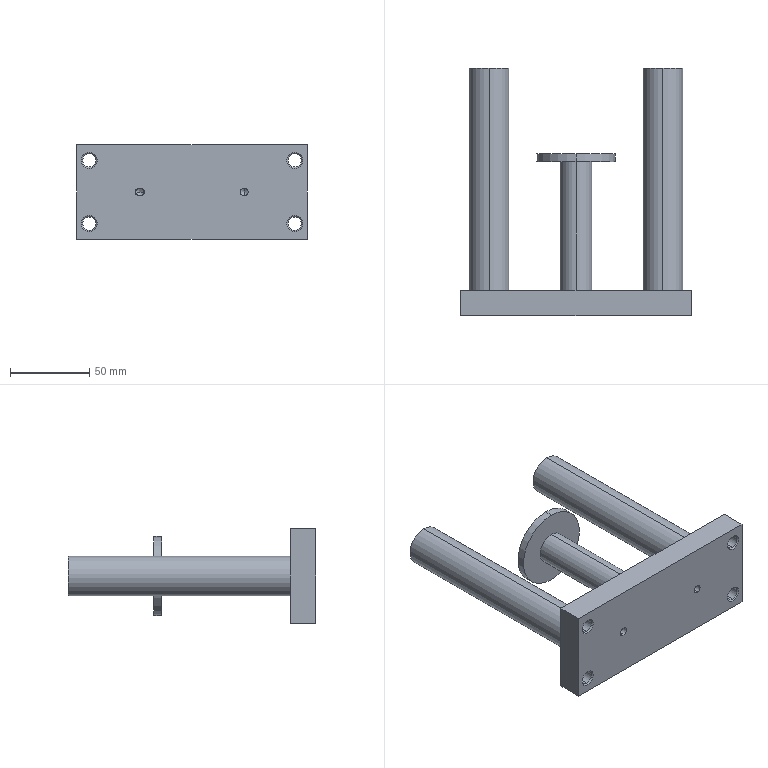Part | SolidWorks | features BaseBody 1 | 1 solid | 56 faces | box 146 x 156.5 x 60 mm | volume 309564 mm3 | cylinder 22 | cone 20 | plane 14 | commonest cylinder face diameters 8.376 x8 5 x6 25 x4 20 x2 50 x2
STEP:
#1=CARTESIAN_POINT('',(33.,107.,140.621));
#2=VERTEX_POINT('',#1);
#3=CARTESIAN_POINT('',(33.,107.,145.621));
#4=VERTEX_POINT('',#3);
#5=CARTESIAN_POINT('',(33.,107.,143.121));
#6=DIRECTION('',(0.,1.,0.));
#7=DIRECTION('',(0.,0.,1.));
#8=AXIS2_PLACEMENT_3D('',#5,#6,#7);
#9=CIRCLE('',#8,2.5);
#10=EDGE_CURVE('',#2,#4,#9,.T.);
#11=ORIENTED_EDGE('',*,*,#10,.F.);
#12=CARTESIAN_POINT('',(33.,115.,140.621));
#13=VERTEX_POINT('',#12);
#14=CARTESIAN_POINT('',(33.,111.,140.621));
#15=DIRECTION('',(0.,1.,0.));
#16=VECTOR('',#15,1000.);
#17=LINE('',#14,#16);
#18=EDGE_CURVE('',#2,#13,#17,.T.);
#19=ORIENTED_EDGE('',*,*,#18,.T.);
#20=CARTESIAN_POINT('',(33.,115.,145.621));
#21=VERTEX_POINT('',#20);
#22=CARTESIAN_POINT('',(33.,115.,143.121));
#23=DIRECTION('',(0.,-1.,0.));
#24=DIRECTION('',(0.,0.,1.));
#25=AXIS2_PLACEMENT_3D('',#22,#23,#24);
#26=CIRCLE('',#25,2.5);
#27=EDGE_CURVE('',#21,#13,#26,.T.);
#28=ORIENTED_EDGE('',*,*,#27,.F.);
#29=CARTESIAN_POINT('',(33.,111.,145.621));
#30=DIRECTION('',(0.,1.,0.));
#31=VECTOR('',#30,1000.);
#32=LINE('',#29,#31);
#33=EDGE_CURVE('',#4,#21,#32,.T.);
#34=ORIENTED_EDGE('',*,*,#33,.F.);
#35=EDGE_LOOP('',(#11,#19,#28,#34));
#36=FACE_OUTER_BOUND('',#35,.T.);
#37=CARTESIAN_POINT('',(33.,111.,143.121));
#38=DIRECTION('',(0.,1.,0.));
#39=DIRECTION('',(0.,0.,1.));
#40=AXIS2_PLACEMENT_3D('',#37,#38,#39);
#41=CYLINDRICAL_SURFACE('',#40,2.5);
#42=ADVANCED_FACE('',(#36),#41,.F.);
#43=CARTESIAN_POINT('',(65.,107.812,127.309));
#44=VERTEX_POINT('',#43);
#45=CARTESIAN_POINT('',(65.,107.812,118.933));
#46=VERTEX_POINT('',#45);
#47=CARTESIAN_POINT('',(65.,107.812,123.121));
#48=DIRECTION('',(0.,-1.,0.));
#49=DIRECTION('',(0.,0.,-1.));
#50=AXIS2_PLACEMENT_3D('',#47,#48,#49);
#51=CIRCLE('',#50,4.188);
#52=EDGE_CURVE('',#44,#46,#51,.T.);
#53=ORIENTED_EDGE('',*,*,#52,.F.);
#54=CARTESIAN_POINT('',(65.,107.,128.121));
#55=VERTEX_POINT('',#54);
#56=CARTESIAN_POINT('',(65.,107.,128.121));
#57=DIRECTION('',(0.,-0.7071,0.7071));
#58=VECTOR('',#57,1000.);
#59=LINE('',#56,#58);
#60=EDGE_CURVE('',#44,#55,#59,.T.);
#61=ORIENTED_EDGE('',*,*,#60,.T.);
#62=CARTESIAN_POINT('',(65.,107.,118.121));
#63=VERTEX_POINT('',#62);
#64=CARTESIAN_POINT('',(65.,107.,123.121));
#65=DIRECTION('',(0.,1.,0.));
#66=DIRECTION('',(0.,0.,-1.));
#67=AXIS2_PLACEMENT_3D('',#64,#65,#66);
#68=CIRCLE('',#67,5.);
#69=EDGE_CURVE('',#63,#55,#68,.T.);
#70=ORIENTED_EDGE('',*,*,#69,.F.);
#71=CARTESIAN_POINT('',(65.,107.,118.121));
#72=DIRECTION('',(0.,-0.7071,-0.7071));
#73=VECTOR('',#72,1000.);
#74=LINE('',#71,#73);
#75=EDGE_CURVE('',#46,#63,#74,.T.);
#76=ORIENTED_EDGE('',*,*,#75,.F.);
#77=EDGE_LOOP('',(#53,#61,#70,#76));
#78=FACE_OUTER_BOUND('',#77,.T.);
#79=CARTESIAN_POINT('',(65.,107.,123.121));
#80=DIRECTION('',(0.,-1.,0.));
#81=DIRECTION('',(0.,0.,-1.));
#82=AXIS2_PLACEMENT_3D('',#79,#80,#81);
#83=CONICAL_SURFACE('',#82,5.,0.7854);
#84=ADVANCED_FACE('',(#78),#83,.F.);
#85=CARTESIAN_POINT('',(65.,107.812,167.309));
#86=VERTEX_POINT('',#85);
#87=CARTESIAN_POINT('',(65.,107.812,158.933));
#88=VERTEX_POINT('',#87);
#89=CARTESIAN_POINT('',(65.,107.812,163.121));
#90=DIRECTION('',(0.,-1.,0.));
#91=DIRECTION('',(0.,0.,-1.));
#92=AXIS2_PLACEMENT_3D('',#89,#90,#91);
#93=CIRCLE('',#92,4.188);
#94=EDGE_CURVE('',#86,#88,#93,.T.);
#95=ORIENTED_EDGE('',*,*,#94,.F.);
#96=CARTESIAN_POINT('',(65.,107.,168.121));
#97=VERTEX_POINT('',#96);
#98=CARTESIAN_POINT('',(65.,107.,168.121));
#99=DIRECTION('',(0.,-0.7071,0.7071));
#100=VECTOR('',#99,1000.);
#101=LINE('',#98,#100);
#102=EDGE_CURVE('',#86,#97,#101,.T.);
#103=ORIENTED_EDGE('',*,*,#102,.T.);
#104=CARTESIAN_POINT('',(65.,107.,158.121));
#105=VERTEX_POINT('',#104);
#106=CARTESIAN_POINT('',(65.,107.,163.121));
#107=DIRECTION('',(0.,1.,0.));
#108=DIRECTION('',(0.,0.,-1.));
#109=AXIS2_PLACEMENT_3D('',#106,#107,#108);
#110=CIRCLE('',#109,5.);
#111=EDGE_CURVE('',#105,#97,#110,.T.);
#112=ORIENTED_EDGE('',*,*,#111,.F.);
#113=CARTESIAN_POINT('',(65.,107.,158.121));
#114=DIRECTION('',(0.,-0.7071,-0.7071));
#115=VECTOR('',#114,1000.);
#116=LINE('',#113,#115);
#117=EDGE_CURVE('',#88,#105,#116,.T.);
#118=ORIENTED_EDGE('',*,*,#117,.F.);
#119=EDGE_LOOP('',(#95,#103,#112,#118));
#120=FACE_OUTER_BOUND('',#119,.T.);
#121=CARTESIAN_POINT('',(65.,107.,163.121));
#122=DIRECTION('',(0.,-1.,0.));
#123=DIRECTION('',(0.,0.,-1.));
#124=AXIS2_PLACEMENT_3D('',#121,#122,#123);
#125=CONICAL_SURFACE('',#124,5.,0.7854);
#126=ADVANCED_FACE('',(#120),#125,.F.);
#127=CARTESIAN_POINT('',(-65.,107.812,167.309));
#128=VERTEX_POINT('',#127);
#129=CARTESIAN_POINT('',(-65.,107.812,158.933));
#130=VERTEX_POINT('',#129);
#131=CARTESIAN_POINT('',(-65.,107.812,163.121));
#132=DIRECTION('',(0.,-1.,0.));
#133=DIRECTION('',(0.,0.,-1.));
#134=AXIS2_PLACEMENT_3D('',#131,#132,#133);
#135=CIRCLE('',#134,4.188);
#136=EDGE_CURVE('',#128,#130,#135,.T.);
#137=ORIENTED_EDGE('',*,*,#136,.F.);
#138=CARTESIAN_POINT('',(-65.,107.,168.121));
#139=VERTEX_POINT('',#138);
#140=CARTESIAN_POINT('',(-65.,107.,168.121));
#141=DIRECTION('',(0.,-0.7071,0.7071));
#142=VECTOR('',#141,1000.);
#143=LINE('',#140,#142);
#144=EDGE_CURVE('',#128,#139,#143,.T.);
#145=ORIENTED_EDGE('',*,*,#144,.T.);
#146=CARTESIAN_POINT('',(-65.,107.,158.121));
#147=VERTEX_POINT('',#146);
#148=CARTESIAN_POINT('',(-65.,107.,163.121));
#149=DIRECTION('',(0.,1.,0.));
#150=DIRECTION('',(0.,0.,-1.));
#151=AXIS2_PLACEMENT_3D('',#148,#149,#150);
#152=CIRCLE('',#151,5.);
#153=EDGE_CURVE('',#147,#139,#152,.T.);
#154=ORIENTED_EDGE('',*,*,#153,.F.);
#155=CARTESIAN_POINT('',(-65.,107.,158.121));
#156=DIRECTION('',(0.,-0.7071,-0.7071));
#157=VECTOR('',#156,1000.);
#158=LINE('',#155,#157);
#159=EDGE_CURVE('',#130,#147,#158,.T.);
#160=ORIENTED_EDGE('',*,*,#159,.F.);
#161=EDGE_LOOP('',(#137,#145,#154,#160));
#162=FACE_OUTER_BOUND('',#161,.T.);
#163=CARTESIAN_POINT('',(-65.,107.,163.121));
#164=DIRECTION('',(0.,-1.,0.));
#165=DIRECTION('',(0.,0.,-1.));
#166=AXIS2_PLACEMENT_3D('',#163,#164,#165);
#167=CONICAL_SURFACE('',#166,5.,0.7854);
#168=ADVANCED_FACE('',(#162),#167,.F.);
#169=CARTESIAN_POINT('',(-65.,107.812,127.309));
#170=VERTEX_POINT('',#169);
#171=CARTESIAN_POINT('',(-65.,107.812,118.933));
#172=VERTEX_POINT('',#171);
#173=CARTESIAN_POINT('',(-65.,107.812,123.121));
#174=DIRECTION('',(0.,-1.,0.));
#175=DIRECTION('',(0.,0.,-1.));
#176=AXIS2_PLACEMENT_3D('',#173,#174,#175);
#177=CIRCLE('',#176,4.188);
#178=EDGE_CURVE('',#170,#172,#177,.T.);
#179=ORIENTED_EDGE('',*,*,#178,.F.);
#180=CARTESIAN_POINT('',(-65.,107.,128.121));
#181=VERTEX_POINT('',#180);
#182=CARTESIAN_POINT('',(-65.,107.,128.121));
#183=DIRECTION('',(0.,-0.7071,0.7071));
#184=VECTOR('',#183,1000.);
#185=LINE('',#182,#184);
#186=EDGE_CURVE('',#170,#181,#185,.T.);
#187=ORIENTED_EDGE('',*,*,#186,.T.);
#188=CARTESIAN_POINT('',(-65.,107.,118.121));
#189=VERTEX_POINT('',#188);
#190=CARTESIAN_POINT('',(-65.,107.,123.121));
#191=DIRECTION('',(0.,1.,0.));
#192=DIRECTION('',(0.,0.,-1.));
#193=AXIS2_PLACEMENT_3D('',#190,#191,#192);
#194=CIRCLE('',#193,5.);
#195=EDGE_CURVE('',#189,#181,#194,.T.);
#196=ORIENTED_EDGE('',*,*,#195,.F.);
#197=CARTESIAN_POINT('',(-65.,107.,118.121));
#198=DIRECTION('',(0.,-0.7071,-0.7071));
#199=VECTOR('',#198,1000.);
#200=LINE('',#197,#199);
#201=EDGE_CURVE('',#172,#189,#200,.T.);
#202=ORIENTED_EDGE('',*,*,#201,.F.);
#203=EDGE_LOOP('',(#179,#187,#196,#202));
#204=FACE_OUTER_BOUND('',#203,.T.);
#205=CARTESIAN_POINT('',(-65.,107.,123.121));
#206=DIRECTION('',(0.,-1.,0.));
#207=DIRECTION('',(0.,0.,-1.));
#208=AXIS2_PLACEMENT_3D('',#205,#206,#207);
#209=CONICAL_SURFACE('',#208,5.,0.7854);
#210=ADVANCED_FACE('',(#204),#209,.F.);
#211=CARTESIAN_POINT('',(33.,116.443,143.121));
#212=VERTEX_POINT('',#211);
#213=CARTESIAN_POINT('',(33.,115.,140.621));
#214=DIRECTION('',(0.,-0.5,-0.866));
#215=VECTOR('',#214,1000.);
#216=LINE('',#213,#215);
#217=EDGE_CURVE('',#212,#13,#216,.T.);
#218=ORIENTED_EDGE('',*,*,#217,.F.);
#219=CARTESIAN_POINT('',(33.,115.,145.621));
#220=DIRECTION('',(0.,-0.5,0.866));
#221=VECTOR('',#220,1000.);
#222=LINE('',#219,#221);
#223=EDGE_CURVE('',#212,#21,#222,.T.);
#224=ORIENTED_EDGE('',*,*,#223,.T.);
#225=ORIENTED_EDGE('',*,*,#27,.T.);
#226=EDGE_LOOP('',(#218,#224,#225));
#227=FACE_OUTER_BOUND('',#226,.T.);
#228=CARTESIAN_POINT('',(33.,115.,143.121));
#229=DIRECTION('',(0.,-1.,0.));
#230=DIRECTION('',(0.,0.,-1.));
#231=AXIS2_PLACEMENT_3D('',#228,#229,#230);
#232=CONICAL_SURFACE('',#231,2.5,1.047);
#233=ADVANCED_FACE('',(#227),#232,.F.);
#234=ORIENTED_EDGE('',*,*,#52,.T.);
#235=CARTESIAN_POINT('',(65.,122.188,118.933));
#236=VERTEX_POINT('',#235);
#237=CARTESIAN_POINT('',(65.,115.,118.933));
#238=DIRECTION('',(0.,1.,0.));
#239=VECTOR('',#238,1000.);
#240=LINE('',#237,#239);
#241=EDGE_CURVE('',#46,#236,#240,.T.);
#242=ORIENTED_EDGE('',*,*,#241,.T.);
#243=CARTESIAN_POINT('',(65.,122.188,127.309));
#244=VERTEX_POINT('',#243);
#245=CARTESIAN_POINT('',(65.,122.188,123.121));
#246=DIRECTION('',(0.,-1.,0.));
#247=DIRECTION('',(0.,0.,1.));
#248=AXIS2_PLACEMENT_3D('',#245,#246,#247);
#249=CIRCLE('',#248,4.188);
#250=EDGE_CURVE('',#244,#236,#249,.T.);
#251=ORIENTED_EDGE('',*,*,#250,.F.);
#252=CARTESIAN_POINT('',(65.,115.,127.309));
#253=DIRECTION('',(0.,1.,0.));
#254=VECTOR('',#253,1000.);
#255=LINE('',#252,#254);
#256=EDGE_CURVE('',#44,#244,#255,.T.);
#257=ORIENTED_EDGE('',*,*,#256,.F.);
#258=EDGE_LOOP('',(#234,#242,#251,#257));
#259=FACE_OUTER_BOUND('',#258,.T.);
#260=CARTESIAN_POINT('',(65.,115.,123.121));
#261=DIRECTION('',(0.,1.,0.));
#262=DIRECTION('',(0.,0.,1.));
#263=AXIS2_PLACEMENT_3D('',#260,#261,#262);
#264=CYLINDRICAL_SURFACE('',#263,4.188);
#265=ADVANCED_FACE('',(#259),#264,.F.);
#266=ORIENTED_EDGE('',*,*,#94,.T.);
#267=CARTESIAN_POINT('',(65.,122.188,158.933));
#268=VERTEX_POINT('',#267);
#269=CARTESIAN_POINT('',(65.,115.,158.933));
#270=DIRECTION('',(0.,1.,0.));
#271=VECTOR('',#270,1000.);
#272=LINE('',#269,#271);
#273=EDGE_CURVE('',#88,#268,#272,.T.);
#274=ORIENTED_EDGE('',*,*,#273,.T.);
#275=CARTESIAN_POINT('',(65.,122.188,167.309));
#276=VERTEX_POINT('',#275);
#277=CARTESIAN_POINT('',(65.,122.188,163.121));
#278=DIRECTION('',(0.,-1.,0.));
#279=DIRECTION('',(0.,0.,1.));
#280=AXIS2_PLACEMENT_3D('',#277,#278,#279);
#281=CIRCLE('',#280,4.188);
#282=EDGE_CURVE('',#276,#268,#281,.T.);
#283=ORIENTED_EDGE('',*,*,#282,.F.);
#284=CARTESIAN_POINT('',(65.,115.,167.309));
#285=DIRECTION('',(0.,1.,0.));
#286=VECTOR('',#285,1000.);
#287=LINE('',#284,#286);
#288=EDGE_CURVE('',#86,#276,#287,.T.);
#289=ORIENTED_EDGE('',*,*,#288,.F.);
#290=EDGE_LOOP('',(#266,#274,#283,#289));
#291=FACE_OUTER_BOUND('',#290,.T.);
#292=CARTESIAN_POINT('',(65.,115.,163.121));
#293=DIRECTION('',(0.,1.,0.));
#294=DIRECTION('',(0.,0.,1.));
#295=AXIS2_PLACEMENT_3D('',#292,#293,#294);
#296=CYLINDRICAL_SURFACE('',#295,4.188);
#297=ADVANCED_FACE('',(#291),#296,.F.);
#298=ORIENTED_EDGE('',*,*,#136,.T.);
#299=CARTESIAN_POINT('',(-65.,122.188,158.933));
#300=VERTEX_POINT('',#299);
#301=CARTESIAN_POINT('',(-65.,115.,158.933));
#302=DIRECTION('',(0.,1.,0.));
#303=VECTOR('',#302,1000.);
#304=LINE('',#301,#303);
#305=EDGE_CURVE('',#130,#300,#304,.T.);
#306=ORIENTED_EDGE('',*,*,#305,.T.);
#307=CARTESIAN_POINT('',(-65.,122.188,167.309));
#308=VERTEX_POINT('',#307);
#309=CARTESIAN_POINT('',(-65.,122.188,163.121));
#310=DIRECTION('',(0.,-1.,0.));
#311=DIRECTION('',(0.,0.,1.));
#312=AXIS2_PLACEMENT_3D('',#309,#310,#311);
#313=CIRCLE('',#312,4.188);
#314=EDGE_CURVE('',#308,#300,#313,.T.);
#315=ORIENTED_EDGE('',*,*,#314,.F.);
#316=CARTESIAN_POINT('',(-65.,115.,167.309));
#317=DIRECTION('',(0.,1.,0.));
#318=VECTOR('',#317,1000.);
#319=LINE('',#316,#318);
#320=EDGE_CURVE('',#128,#308,#319,.T.);
#321=ORIENTED_EDGE('',*,*,#320,.F.);
#322=EDGE_LOOP('',(#298,#306,#315,#321));
#323=FACE_OUTER_BOUND('',#322,.T.);
#324=CARTESIAN_POINT('',(-65.,115.,163.121));
#325=DIRECTION('',(0.,1.,0.));
#326=DIRECTION('',(0.,0.,1.));
#327=AXIS2_PLACEMENT_3D('',#324,#325,#326);
#328=CYLINDRICAL_SURFACE('',#327,4.188);
#329=ADVANCED_FACE('',(#323),#328,.F.);
#330=ORIENTED_EDGE('',*,*,#178,.T.);
#331=CARTESIAN_POINT('',(-65.,122.188,118.933));
#332=VERTEX_POINT('',#331);
#333=CARTESIAN_POINT('',(-65.,115.,118.933));
#334=DIRECTION('',(0.,1.,0.));
#335=VECTOR('',#334,1000.);
#336=LINE('',#333,#335);
#337=EDGE_CURVE('',#172,#332,#336,.T.);
#338=ORIENTED_EDGE('',*,*,#337,.T.);
#339=CARTESIAN_POINT('',(-65.,122.188,127.309));
#340=VERTEX_POINT('',#339);
#341=CARTESIAN_POINT('',(-65.,122.188,123.121));
#342=DIRECTION('',(0.,-1.,0.));
#343=DIRECTION('',(0.,0.,1.));
#344=AXIS2_PLACEMENT_3D('',#341,#342,#343);
#345=CIRCLE('',#344,4.188);
#346=EDGE_CURVE('',#340,#332,#345,.T.);
#347=ORIENTED_EDGE('',*,*,#346,.F.);
#348=CARTESIAN_POINT('',(-65.,115.,127.309));
#349=DIRECTION('',(0.,1.,0.));
#350=VECTOR('',#349,1000.);
#351=LINE('',#348,#350);
#352=EDGE_CURVE('',#170,#340,#351,.T.);
#353=ORIENTED_EDGE('',*,*,#352,.F.);
#354=EDGE_LOOP('',(#330,#338,#347,#353));
#355=FACE_OUTER_BOUND('',#354,.T.);
#356=CARTESIAN_POINT('',(-65.,115.,123.121));
#357=DIRECTION('',(0.,1.,0.));
#358=DIRECTION('',(0.,0.,1.));
#359=AXIS2_PLACEMENT_3D('',#356,#357,#358);
#360=CYLINDRICAL_SURFACE('',#359,4.188);
#361=ADVANCED_FACE('',(#355),#360,.F.);
#362=CARTESIAN_POINT('',(-33.,111.,140.621));
#363=VERTEX_POINT('',#362);
#364=CARTESIAN_POINT('',(-33.,111.,145.621));
#365=VERTEX_POINT('',#364);
#366=CARTESIAN_POINT('',(-33.,111.,143.121));
#367=DIRECTION('',(0.,1.,0.));
#368=DIRECTION('',(0.,0.,1.));
#369=AXIS2_PLACEMENT_3D('',#366,#367,#368);
#370=CIRCLE('',#369,2.5);
#371=EDGE_CURVE('',#363,#365,#370,.T.);
#372=ORIENTED_EDGE('',*,*,#371,.F.);
#373=CARTESIAN_POINT('',(-33.,115.,140.621));
#374=VERTEX_POINT('',#373);
#375=CARTESIAN_POINT('',(-33.,111.,140.621));
#376=DIRECTION('',(0.,1.,0.));
#377=VECTOR('',#376,1000.);
#378=LINE('',#375,#377);
#379=EDGE_CURVE('',#363,#374,#378,.T.);
#380=ORIENTED_EDGE('',*,*,#379,.T.);
#381=CARTESIAN_POINT('',(-35.5,115.,143.121));
#382=VERTEX_POINT('',#381);
#383=CARTESIAN_POINT('',(-33.,115.,143.121));
#384=DIRECTION('',(0.,-1.,0.));
#385=DIRECTION('',(0.,0.,1.));
#386=AXIS2_PLACEMENT_3D('',#383,#384,#385);
#387=CIRCLE('',#386,2.5);
#388=EDGE_CURVE('',#382,#374,#387,.T.);
#389=ORIENTED_EDGE('',*,*,#388,.F.);
#390=CARTESIAN_POINT('',(-33.,115.,145.621));
#391=VERTEX_POINT('',#390);
#392=CARTESIAN_POINT('',(-33.,115.,143.121));
#393=DIRECTION('',(0.,-1.,0.));
#394=DIRECTION('',(0.,0.,1.));
#395=AXIS2_PLACEMENT_3D('',#392,#393,#394);
#396=CIRCLE('',#395,2.5);
#397=EDGE_CURVE('',#391,#382,#396,.T.);
#398=ORIENTED_EDGE('',*,*,#397,.F.);
#399=CARTESIAN_POINT('',(-33.,111.,145.621));
#400=DIRECTION('',(0.,1.,0.));
#401=VECTOR('',#400,1000.);
#402=LINE('',#399,#401);
#403=EDGE_CURVE('',#365,#391,#402,.T.);
#404=ORIENTED_EDGE('',*,*,#403,.F.);
#405=EDGE_LOOP('',(#372,#380,#389,#398,#404));
#406=FACE_OUTER_BOUND('',#405,.T.);
#407=CARTESIAN_POINT('',(-33.,111.,143.121));
#408=DIRECTION('',(0.,1.,0.));
#409=DIRECTION('',(0.,0.,1.));
#410=AXIS2_PLACEMENT_3D('',#407,#408,#409);
#411=CYLINDRICAL_SURFACE('',#410,2.5);
#412=ADVANCED_FACE('',(#406),#411,.F.);
#413=ORIENTED_EDGE('',*,*,#250,.T.);
#414=CARTESIAN_POINT('',(65.,123.,118.121));
#415=VERTEX_POINT('',#414);
#416=CARTESIAN_POINT('',(65.,123.,118.121));
#417=DIRECTION('',(0.,0.7071,-0.7071));
#418=VECTOR('',#417,1000.);
#419=LINE('',#416,#418);
#420=EDGE_CURVE('',#236,#415,#419,.T.);
#421=ORIENTED_EDGE('',*,*,#420,.T.);
#422=CARTESIAN_POINT('',(65.,123.,128.121));
#423=VERTEX_POINT('',#422);
#424=CARTESIAN_POINT('',(65.,123.,123.121));
#425=DIRECTION('',(0.,1.,0.));
#426=DIRECTION('',(0.,0.,1.));
#427=AXIS2_PLACEMENT_3D('',#424,#425,#426);
#428=CIRCLE('',#427,5.);
#429=EDGE_CURVE('',#415,#423,#428,.T.);
#430=ORIENTED_EDGE('',*,*,#429,.T.);
#431=CARTESIAN_POINT('',(65.,123.,128.121));
#432=DIRECTION('',(0.,0.7071,0.7071));
#433=VECTOR('',#432,1000.);
#434=LINE('',#431,#433);
#435=EDGE_CURVE('',#244,#423,#434,.T.);
#436=ORIENTED_EDGE('',*,*,#435,.F.);
#437=EDGE_LOOP('',(#413,#421,#430,#436));
#438=FACE_OUTER_BOUND('',#437,.T.);
#439=CARTESIAN_POINT('',(65.,123.,123.121));
#440=DIRECTION('',(0.,1.,0.));
#441=DIRECTION('',(0.,0.,1.));
#442=AXIS2_PLACEMENT_3D('',#439,#440,#441);
#443=CONICAL_SURFACE('',#442,5.,0.7854);
#444=ADVANCED_FACE('',(#438),#443,.F.);
#445=ORIENTED_EDGE('',*,*,#282,.T.);
#446=CARTESIAN_POINT('',(65.,123.,158.121));
#447=VERTEX_POINT('',#446);
#448=CARTESIAN_POINT('',(65.,123.,158.121));
#449=DIRECTION('',(0.,0.7071,-0.7071));
#450=VECTOR('',#449,1000.);
#451=LINE('',#448,#450);
#452=EDGE_CURVE('',#268,#447,#451,.T.);
#453=ORIENTED_EDGE('',*,*,#452,.T.);
#454=CARTESIAN_POINT('',(65.,123.,168.121));
#455=VERTEX_POINT('',#454);
#456=CARTESIAN_POINT('',(65.,123.,163.121));
#457=DIRECTION('',(0.,1.,0.));
#458=DIRECTION('',(0.,0.,1.));
#459=AXIS2_PLACEMENT_3D('',#456,#457,#458);
#460=CIRCLE('',#459,5.);
#461=EDGE_CURVE('',#447,#455,#460,.T.);
#462=ORIENTED_EDGE('',*,*,#461,.T.);
#463=CARTESIAN_POINT('',(65.,123.,168.121));
#464=DIRECTION('',(0.,0.7071,0.7071));
#465=VECTOR('',#464,1000.);
#466=LINE('',#463,#465);
#467=EDGE_CURVE('',#276,#455,#466,.T.);
#468=ORIENTED_EDGE('',*,*,#467,.F.);
#469=EDGE_LOOP('',(#445,#453,#462,#468));
#470=FACE_OUTER_BOUND('',#469,.T.);
#471=CARTESIAN_POINT('',(65.,123.,163.121));
#472=DIRECTION('',(0.,1.,0.));
#473=DIRECTION('',(0.,0.,1.));
#474=AXIS2_PLACEMENT_3D('',#471,#472,#473);
#475=CONICAL_SURFACE('',#474,5.,0.7854);
#476=ADVANCED_FACE('',(#470),#475,.F.);
#477=ORIENTED_EDGE('',*,*,#314,.T.);
#478=CARTESIAN_POINT('',(-65.,123.,158.121));
#479=VERTEX_POINT('',#478);
#480=CARTESIAN_POINT('',(-65.,123.,158.121));
#481=DIRECTION('',(0.,0.7071,-0.7071));
#482=VECTOR('',#481,1000.);
#483=LINE('',#480,#482);
#484=EDGE_CURVE('',#300,#479,#483,.T.);
#485=ORIENTED_EDGE('',*,*,#484,.T.);
#486=CARTESIAN_POINT('',(-65.,123.,168.121));
#487=VERTEX_POINT('',#486);
#488=CARTESIAN_POINT('',(-65.,123.,163.121));
#489=DIRECTION('',(0.,1.,0.));
#490=DIRECTION('',(0.,0.,1.));
#491=AXIS2_PLACEMENT_3D('',#488,#489,#490);
#492=CIRCLE('',#491,5.);
#493=EDGE_CURVE('',#479,#487,#492,.T.);
#494=ORIENTED_EDGE('',*,*,#493,.T.);
#495=CARTESIAN_POINT('',(-65.,123.,168.121));
#496=DIRECTION('',(0.,0.7071,0.7071));
#497=VECTOR('',#496,1000.);
#498=LINE('',#495,#497);
#499=EDGE_CURVE('',#308,#487,#498,.T.);
#500=ORIENTED_EDGE('',*,*,#499,.F.);
#501=EDGE_LOOP('',(#477,#485,#494,#500));
#502=FACE_OUTER_BOUND('',#501,.T.);
#503=CARTESIAN_POINT('',(-65.,123.,163.121));
#504=DIRECTION('',(0.,1.,0.));
#505=DIRECTION('',(0.,0.,1.));
#506=AXIS2_PLACEMENT_3D('',#503,#504,#505);
#507=CONICAL_SURFACE('',#506,5.,0.7854);
#508=ADVANCED_FACE('',(#502),#507,.F.);
#509=ORIENTED_EDGE('',*,*,#346,.T.);
#510=CARTESIAN_POINT('',(-65.,123.,118.121));
#511=VERTEX_POINT('',#510);
#512=CARTESIAN_POINT('',(-65.,123.,118.121));
#513=DIRECTION('',(0.,0.7071,-0.7071));
#514=VECTOR('',#513,1000.);
#515=LINE('',#512,#514);
#516=EDGE_CURVE('',#332,#511,#515,.T.);
#517=ORIENTED_EDGE('',*,*,#516,.T.);
#518=CARTESIAN_POINT('',(-65.,123.,128.121));
#519=VERTEX_POINT('',#518);
#520=CARTESIAN_POINT('',(-65.,123.,123.121));
#521=DIRECTION('',(0.,1.,0.));
#522=DIRECTION('',(0.,0.,1.));
#523=AXIS2_PLACEMENT_3D('',#520,#521,#522);
#524=CIRCLE('',#523,5.);
#525=EDGE_CURVE('',#511,#519,#524,.T.);
#526=ORIENTED_EDGE('',*,*,#525,.T.);
#527=CARTESIAN_POINT('',(-65.,123.,128.121));
#528=DIRECTION('',(0.,0.7071,0.7071));
#529=VECTOR('',#528,1000.);
#530=LINE('',#527,#529);
#531=EDGE_CURVE('',#340,#519,#530,.T.);
#532=ORIENTED_EDGE('',*,*,#531,.F.);
#533=EDGE_LOOP('',(#509,#517,#526,#532));
#534=FACE_OUTER_BOUND('',#533,.T.);
#535=CARTESIAN_POINT('',(-65.,123.,123.121));
#536=DIRECTION('',(0.,1.,0.));
#537=DIRECTION('',(0.,0.,1.));
#538=AXIS2_PLACEMENT_3D('',#535,#536,#537);
#539=CONICAL_SURFACE('',#538,5.,0.7854);
#540=ADVANCED_FACE('',(#534),#539,.F.);
#541=CARTESIAN_POINT('',(0.,204.5,133.121));
#542=VERTEX_POINT('',#541);
#543=CARTESIAN_POINT('',(0.,204.5,153.121));
#544=VERTEX_POINT('',#543);
#545=CARTESIAN_POINT('',(0.,204.5,143.121));
#546=DIRECTION('',(0.,-1.,0.));
#547=DIRECTION('',(0.,0.,-1.));
#548=AXIS2_PLACEMENT_3D('',#545,#546,#547);
#549=CIRCLE('',#548,10.);
#550=EDGE_CURVE('',#542,#544,#549,.T.);
#551=ORIENTED_EDGE('',*,*,#550,.T.);
#552=CARTESIAN_POINT('',(0.,123.,153.121));
#553=VERTEX_POINT('',#552);
#554=CARTESIAN_POINT('',(0.,123.,153.121));
#555=DIRECTION('',(0.,-1.,0.));
#556=VECTOR('',#555,1000.);
#557=LINE('',#554,#556);
#558=EDGE_CURVE('',#544,#553,#557,.T.);
#559=ORIENTED_EDGE('',*,*,#558,.T.);
#560=CARTESIAN_POINT('',(0.,123.,133.121));
#561=VERTEX_POINT('',#560);
#562=CARTESIAN_POINT('',(0.,123.,143.121));
#563=DIRECTION('',(0.,1.,0.));
#564=DIRECTION('',(0.,0.,-1.));
#565=AXIS2_PLACEMENT_3D('',#562,#563,#564);
#566=CIRCLE('',#565,10.);
#567=EDGE_CURVE('',#553,#561,#566,.T.);
#568=ORIENTED_EDGE('',*,*,#567,.T.);
#569=CARTESIAN_POINT('',(0.,123.,133.121));
#570=DIRECTION('',(0.,-1.,0.));
#571=VECTOR('',#570,1000.);
#572=LINE('',#569,#571);
#573=EDGE_CURVE('',#542,#561,#572,.T.);
#574=ORIENTED_EDGE('',*,*,#573,.F.);
#575=EDGE_LOOP('',(#551,#559,#568,#574));
#576=FACE_OUTER_BOUND('',#575,.T.);
#577=CARTESIAN_POINT('',(0.,123.,143.121));
#578=DIRECTION('',(0.,-1.,0.));
#579=DIRECTION('',(0.,0.,-1.));
#580=AXIS2_PLACEMENT_3D('',#577,#578,#579);
#581=CYLINDRICAL_SURFACE('',#580,10.);
#582=ADVANCED_FACE('',(#576),#581,.T.);
#583=CARTESIAN_POINT('',(55.,263.5,130.621));
#584=VERTEX_POINT('',#583);
#585=CARTESIAN_POINT('',(55.,263.5,155.621));
#586=VERTEX_POINT('',#585);
#587=CARTESIAN_POINT('',(55.,263.5,143.121));
#588=DIRECTION('',(0.,-1.,0.));
#589=DIRECTION('',(0.,0.,-1.));
#590=AXIS2_PLACEMENT_3D('',#587,#588,#589);
#591=CIRCLE('',#590,12.5);
#592=EDGE_CURVE('',#584,#586,#591,.T.);
#593=ORIENTED_EDGE('',*,*,#592,.T.);
#594=CARTESIAN_POINT('',(55.,123.,155.621));
#595=VERTEX_POINT('',#594);
#596=CARTESIAN_POINT('',(55.,123.,155.621));
#597=DIRECTION('',(0.,-1.,0.));
#598=VECTOR('',#597,1000.);
#599=LINE('',#596,#598);
#600=EDGE_CURVE('',#586,#595,#599,.T.);
#601=ORIENTED_EDGE('',*,*,#600,.T.);
#602=CARTESIAN_POINT('',(55.,123.,130.621));
#603=VERTEX_POINT('',#602);
#604=CARTESIAN_POINT('',(55.,123.,143.121));
#605=DIRECTION('',(0.,1.,0.));
#606=DIRECTION('',(0.,0.,-1.));
#607=AXIS2_PLACEMENT_3D('',#604,#605,#606);
#608=CIRCLE('',#607,12.5);
#609=EDGE_CURVE('',#595,#603,#608,.T.);
#610=ORIENTED_EDGE('',*,*,#609,.T.);
#611=CARTESIAN_POINT('',(55.,123.,130.621));
#612=DIRECTION('',(0.,-1.,0.));
#613=VECTOR('',#612,1000.);
#614=LINE('',#611,#613);
#615=EDGE_CURVE('',#584,#603,#614,.T.);
#616=ORIENTED_EDGE('',*,*,#615,.F.);
#617=EDGE_LOOP('',(#593,#601,#610,#616));
#618=FACE_OUTER_BOUND('',#617,.T.);
#619=CARTESIAN_POINT('',(55.,123.,143.121));
#620=DIRECTION('',(0.,-1.,0.));
#621=DIRECTION('',(0.,0.,-1.));
#622=AXIS2_PLACEMENT_3D('',#619,#620,#621);
#623=CYLINDRICAL_SURFACE('',#622,12.5);
#624=ADVANCED_FACE('',(#618),#623,.T.);
#625=CARTESIAN_POINT('',(-55.,263.5,130.621));
#626=VERTEX_POINT('',#625);
#627=CARTESIAN_POINT('',(-55.,263.5,155.621));
#628=VERTEX_POINT('',#627);
#629=CARTESIAN_POINT('',(-55.,263.5,143.121));
#630=DIRECTION('',(0.,-1.,0.));
#631=DIRECTION('',(0.,0.,-1.));
#632=AXIS2_PLACEMENT_3D('',#629,#630,#631);
#633=CIRCLE('',#632,12.5);
#634=EDGE_CURVE('',#626,#628,#633,.T.);
#635=ORIENTED_EDGE('',*,*,#634,.T.);
#636=CARTESIAN_POINT('',(-55.,123.,155.621));
#637=VERTEX_POINT('',#636);
#638=CARTESIAN_POINT('',(-55.,123.,155.621));
#639=DIRECTION('',(0.,-1.,0.));
#640=VECTOR('',#639,1000.);
#641=LINE('',#638,#640);
#642=EDGE_CURVE('',#628,#637,#641,.T.);
#643=ORIENTED_EDGE('',*,*,#642,.T.);
#644=CARTESIAN_POINT('',(-55.,123.,130.621));
#645=VERTEX_POINT('',#644);
#646=CARTESIAN_POINT('',(-55.,123.,143.121));
#647=DIRECTION('',(0.,1.,0.));
#648=DIRECTION('',(0.,0.,-1.));
#649=AXIS2_PLACEMENT_3D('',#646,#647,#648);
#650=CIRCLE('',#649,12.5);
#651=EDGE_CURVE('',#637,#645,#650,.T.);
#652=ORIENTED_EDGE('',*,*,#651,.T.);
#653=CARTESIAN_POINT('',(-55.,123.,130.621));
#654=DIRECTION('',(0.,-1.,0.));
#655=VECTOR('',#654,1000.);
#656=LINE('',#653,#655);
#657=EDGE_CURVE('',#626,#645,#656,.T.);
#658=ORIENTED_EDGE('',*,*,#657,.F.);
#659=EDGE_LOOP('',(#635,#643,#652,#658));
#660=FACE_OUTER_BOUND('',#659,.T.);
#661=CARTESIAN_POINT('',(-55.,123.,143.121));
#662=DIRECTION('',(0.,-1.,0.));
#663=DIRECTION('',(0.,0.,-1.));
#664=AXIS2_PLACEMENT_3D('',#661,#662,#663);
#665=CYLINDRICAL_SURFACE('',#664,12.5);
#666=ADVANCED_FACE('',(#660),#665,.T.);
#667=CARTESIAN_POINT('',(-33.,116.443,143.121));
#668=VERTEX_POINT('',#667);
#669=CARTESIAN_POINT('',(-30.5,115.,143.121));
#670=VERTEX_POINT('',#669);
#671=CARTESIAN_POINT('',(-30.5,115.,143.121));
#672=DIRECTION('',(0.866,-0.5,0.));
#673=VECTOR('',#672,1000.);
#674=LINE('',#671,#673);
#675=EDGE_CURVE('',#668,#670,#674,.T.);
#676=ORIENTED_EDGE('',*,*,#675,.F.);
#677=CARTESIAN_POINT('',(-35.5,115.,143.121));
#678=DIRECTION('',(-0.866,-0.5,0.));
#679=VECTOR('',#678,1000.);
#680=LINE('',#677,#679);
#681=EDGE_CURVE('',#668,#382,#680,.T.);
#682=ORIENTED_EDGE('',*,*,#681,.T.);
#683=ORIENTED_EDGE('',*,*,#388,.T.);
#684=CARTESIAN_POINT('',(-33.,115.,143.121));
#685=DIRECTION('',(0.,-1.,0.));
#686=DIRECTION('',(0.,0.,1.));
#687=AXIS2_PLACEMENT_3D('',#684,#685,#686);
#688=CIRCLE('',#687,2.5);
#689=EDGE_CURVE('',#374,#670,#688,.T.);
#690=ORIENTED_EDGE('',*,*,#689,.T.);
#691=EDGE_LOOP('',(#676,#682,#683,#690));
#692=FACE_OUTER_BOUND('',#691,.T.);
#693=CARTESIAN_POINT('',(-33.,115.,143.121));
#694=DIRECTION('',(0.,-1.,0.));
#695=DIRECTION('',(1.,0.,0.));
#696=AXIS2_PLACEMENT_3D('',#693,#694,#695);
#697=CONICAL_SURFACE('',#696,2.5,1.047);
#698=ADVANCED_FACE('',(#692),#697,.F.);
#699=CARTESIAN_POINT('',(0.,204.5,118.121));
#700=VERTEX_POINT('',#699);
#701=CARTESIAN_POINT('',(0.,204.5,168.121));
#702=VERTEX_POINT('',#701);
#703=CARTESIAN_POINT('',(0.,204.5,143.121));
#704=DIRECTION('',(0.,-1.,0.));
#705=DIRECTION('',(0.,0.,1.));
#706=AXIS2_PLACEMENT_3D('',#703,#704,#705);
#707=CIRCLE('',#706,25.);
#708=EDGE_CURVE('',#700,#702,#707,.T.);
#709=ORIENTED_EDGE('',*,*,#708,.F.);
#710=CARTESIAN_POINT('',(0.,209.5,118.121));
#711=VERTEX_POINT('',#710);
#712=CARTESIAN_POINT('',(0.,209.5,118.121));
#713=DIRECTION('',(0.,1.,0.));
#714=VECTOR('',#713,1000.);
#715=LINE('',#712,#714);
#716=EDGE_CURVE('',#700,#711,#715,.T.);
#717=ORIENTED_EDGE('',*,*,#716,.T.);
#718=CARTESIAN_POINT('',(0.,209.5,168.121));
#719=VERTEX_POINT('',#718);
#720=CARTESIAN_POINT('',(0.,209.5,143.121));
#721=DIRECTION('',(0.,-1.,0.));
#722=DIRECTION('',(0.,0.,1.));
#723=AXIS2_PLACEMENT_3D('',#720,#721,#722);
#724=CIRCLE('',#723,25.);
#725=EDGE_CURVE('',#711,#719,#724,.T.);
#726=ORIENTED_EDGE('',*,*,#725,.T.);
#727=CARTESIAN_POINT('',(0.,209.5,168.121));
#728=DIRECTION('',(0.,1.,0.));
#729=VECTOR('',#728,1000.);
#730=LINE('',#727,#729);
#731=EDGE_CURVE('',#702,#719,#730,.T.);
#732=ORIENTED_EDGE('',*,*,#731,.F.);
#733=EDGE_LOOP('',(#709,#717,#726,#732));
#734=FACE_OUTER_BOUND('',#733,.T.);
#735=CARTESIAN_POINT('',(0.,209.5,143.121));
#736=DIRECTION('',(0.,1.,0.));
#737=DIRECTION('',(0.,0.,1.));
#738=AXIS2_PLACEMENT_3D('',#735,#736,#737);
#739=CYLINDRICAL_SURFACE('',#738,25.);
#740=ADVANCED_FACE('',(#734),#739,.T.);
#741=CARTESIAN_POINT('',(-32.5,107.,140.621));
#742=VERTEX_POINT('',#741);
#743=CARTESIAN_POINT('',(-33.5,107.,140.621));
#744=VERTEX_POINT('',#743);
#745=CARTESIAN_POINT('',(-33.5,107.,140.621));
#746=DIRECTION('',(-1.,0.,0.));
#747=VECTOR('',#746,1000.);
#748=LINE('',#745,#747);
#749=EDGE_CURVE('',#742,#744,#748,.T.);
#750=ORIENTED_EDGE('',*,*,#749,.T.);
#751=CARTESIAN_POINT('',(-33.5,107.,145.621));
#752=VERTEX_POINT('',#751);
#753=CARTESIAN_POINT('',(-33.5,107.,143.121));
#754=DIRECTION('',(0.,1.,0.));
#755=DIRECTION('',(0.,0.,-1.));
#756=AXIS2_PLACEMENT_3D('',#753,#754,#755);
#757=CIRCLE('',#756,2.5);
#758=EDGE_CURVE('',#744,#752,#757,.T.);
#759=ORIENTED_EDGE('',*,*,#758,.T.);
#760=CARTESIAN_POINT('',(-32.5,107.,145.621));
#761=VERTEX_POINT('',#760);
#762=CARTESIAN_POINT('',(-32.5,107.,145.621));
#763=DIRECTION('',(1.,0.,0.));
#764=VECTOR('',#763,1000.);
#765=LINE('',#762,#764);
#766=EDGE_CURVE('',#752,#761,#765,.T.);
#767=ORIENTED_EDGE('',*,*,#766,.T.);
#768=CARTESIAN_POINT('',(-32.5,107.,143.121));
#769=DIRECTION('',(0.,1.,0.));
#770=DIRECTION('',(0.,0.,-1.));
#771=AXIS2_PLACEMENT_3D('',#768,#769,#770);
#772=CIRCLE('',#771,2.5);
#773=EDGE_CURVE('',#761,#742,#772,.T.);
#774=ORIENTED_EDGE('',*,*,#773,.T.);
#775=EDGE_LOOP('',(#750,#759,#767,#774));
#776=FACE_BOUND('',#775,.T.);
#777=CARTESIAN_POINT('',(33.,107.,143.121));
#778=DIRECTION('',(0.,1.,0.));
#779=DIRECTION('',(0.,0.,1.));
#780=AXIS2_PLACEMENT_3D('',#777,#778,#779);
#781=CIRCLE('',#780,2.5);
#782=EDGE_CURVE('',#4,#2,#781,.T.);
#783=ORIENTED_EDGE('',*,*,#782,.T.);
#784=ORIENTED_EDGE('',*,*,#10,.T.);
#785=EDGE_LOOP('',(#783,#784));
#786=FACE_BOUND('',#785,.T.);
#787=ORIENTED_EDGE('',*,*,#69,.T.);
#788=CARTESIAN_POINT('',(65.,107.,123.121));
#789=DIRECTION('',(0.,1.,0.));
#790=DIRECTION('',(0.,0.,-1.));
#791=AXIS2_PLACEMENT_3D('',#788,#789,#790);
#792=CIRCLE('',#791,5.);
#793=EDGE_CURVE('',#55,#63,#792,.T.);
#794=ORIENTED_EDGE('',*,*,#793,.T.);
#795=EDGE_LOOP('',(#787,#794));
#796=FACE_BOUND('',#795,.T.);
#797=ORIENTED_EDGE('',*,*,#111,.T.);
#798=CARTESIAN_POINT('',(65.,107.,163.121));
#799=DIRECTION('',(0.,1.,0.));
#800=DIRECTION('',(0.,0.,-1.));
#801=AXIS2_PLACEMENT_3D('',#798,#799,#800);
#802=CIRCLE('',#801,5.);
#803=EDGE_CURVE('',#97,#105,#802,.T.);
#804=ORIENTED_EDGE('',*,*,#803,.T.);
#805=EDGE_LOOP('',(#797,#804));
#806=FACE_BOUND('',#805,.T.);
#807=ORIENTED_EDGE('',*,*,#153,.T.);
#808=CARTESIAN_POINT('',(-65.,107.,163.121));
#809=DIRECTION('',(0.,1.,0.));
#810=DIRECTION('',(0.,0.,-1.));
#811=AXIS2_PLACEMENT_3D('',#808,#809,#810);
#812=CIRCLE('',#811,5.);
#813=EDGE_CURVE('',#139,#147,#812,.T.);
#814=ORIENTED_EDGE('',*,*,#813,.T.);
#815=EDGE_LOOP('',(#807,#814));
#816=FACE_BOUND('',#815,.T.);
#817=ORIENTED_EDGE('',*,*,#195,.T.);
#818=CARTESIAN_POINT('',(-65.,107.,123.121));
#819=DIRECTION('',(0.,1.,0.));
#820=DIRECTION('',(0.,0.,-1.));
#821=AXIS2_PLACEMENT_3D('',#818,#819,#820);
#822=CIRCLE('',#821,5.);
#823=EDGE_CURVE('',#181,#189,#822,.T.);
#824=ORIENTED_EDGE('',*,*,#823,.T.);
#825=EDGE_LOOP('',(#817,#824));
#826=FACE_BOUND('',#825,.T.);
#827=CARTESIAN_POINT('',(73.,107.,113.121));
#828=VERTEX_POINT('',#827);
#829=CARTESIAN_POINT('',(73.,107.,173.121));
#830=VERTEX_POINT('',#829);
#831=CARTESIAN_POINT('',(73.,107.,143.121));
#832=DIRECTION('',(0.,0.,1.));
#833=VECTOR('',#832,1000.);
#834=LINE('',#831,#833);
#835=EDGE_CURVE('',#828,#830,#834,.T.);
#836=ORIENTED_EDGE('',*,*,#835,.T.);
#837=CARTESIAN_POINT('',(-73.,107.,173.121));
#838=VERTEX_POINT('',#837);
#839=CARTESIAN_POINT('',(0.,107.,173.121));
#840=DIRECTION('',(-1.,0.,0.));
#841=VECTOR('',#840,1000.);
#842=LINE('',#839,#841);
#843=EDGE_CURVE('',#830,#838,#842,.T.);
#844=ORIENTED_EDGE('',*,*,#843,.T.);
#845=CARTESIAN_POINT('',(-73.,107.,113.121));
#846=VERTEX_POINT('',#845);
#847=CARTESIAN_POINT('',(-73.,107.,143.121));
#848=DIRECTION('',(0.,0.,-1.));
#849=VECTOR('',#848,1000.);
#850=LINE('',#847,#849);
#851=EDGE_CURVE('',#838,#846,#850,.T.);
#852=ORIENTED_EDGE('',*,*,#851,.T.);
#853=CARTESIAN_POINT('',(0.,107.,113.121));
#854=DIRECTION('',(1.,0.,0.));
#855=VECTOR('',#854,1000.);
#856=LINE('',#853,#855);
#857=EDGE_CURVE('',#846,#828,#856,.T.);
#858=ORIENTED_EDGE('',*,*,#857,.T.);
#859=EDGE_LOOP('',(#836,#844,#852,#858));
#860=FACE_OUTER_BOUND('',#859,.T.);
#861=CARTESIAN_POINT('',(0.,107.,143.121));
#862=DIRECTION('',(0.,-1.,0.));
#863=DIRECTION('',(0.,0.,-1.));
#864=AXIS2_PLACEMENT_3D('',#861,#862,#863);
#865=PLANE('',#864);
#866=ADVANCED_FACE('',(#776,#786,#796,#806,#816,#826,#860),#865,.T.);
#867=ORIENTED_EDGE('',*,*,#758,.F.);
#868=CARTESIAN_POINT('',(-33.5,111.,140.621));
#869=VERTEX_POINT('',#868);
#870=CARTESIAN_POINT('',(-33.5,107.,140.621));
#871=DIRECTION('',(0.,-1.,0.));
#872=VECTOR('',#871,1000.);
#873=LINE('',#870,#872);
#874=EDGE_CURVE('',#869,#744,#873,.T.);
#875=ORIENTED_EDGE('',*,*,#874,.F.);
#876=CARTESIAN_POINT('',(-33.5,111.,145.621));
#877=VERTEX_POINT('',#876);
#878=CARTESIAN_POINT('',(-33.5,111.,143.121));
#879=DIRECTION('',(0.,-1.,0.));
#880=DIRECTION('',(0.,0.,-1.));
#881=AXIS2_PLACEMENT_3D('',#878,#879,#880);
#882=CIRCLE('',#881,2.5);
#883=EDGE_CURVE('',#877,#869,#882,.T.);
#884=ORIENTED_EDGE('',*,*,#883,.F.);
#885=CARTESIAN_POINT('',(-33.5,107.,145.621));
#886=DIRECTION('',(0.,1.,0.));
#887=VECTOR('',#886,1000.);
#888=LINE('',#885,#887);
#889=EDGE_CURVE('',#752,#877,#888,.T.);
#890=ORIENTED_EDGE('',*,*,#889,.F.);
#891=EDGE_LOOP('',(#867,#875,#884,#890));
#892=FACE_OUTER_BOUND('',#891,.T.);
#893=CARTESIAN_POINT('',(-33.5,107.,143.121));
#894=DIRECTION('',(0.,-1.,0.));
#895=DIRECTION('',(0.,0.,-1.));
#896=AXIS2_PLACEMENT_3D('',#893,#894,#895);
#897=CYLINDRICAL_SURFACE('',#896,2.5);
#898=ADVANCED_FACE('',(#892),#897,.F.);
#899=ORIENTED_EDGE('',*,*,#773,.F.);
#900=CARTESIAN_POINT('',(-32.5,111.,145.621));
#901=VERTEX_POINT('',#900);
#902=CARTESIAN_POINT('',(-32.5,107.,145.621));
#903=DIRECTION('',(0.,-1.,0.));
#904=VECTOR('',#903,1000.);
#905=LINE('',#902,#904);
#906=EDGE_CURVE('',#901,#761,#905,.T.);
#907=ORIENTED_EDGE('',*,*,#906,.F.);
#908=CARTESIAN_POINT('',(-32.5,111.,140.621));
#909=VERTEX_POINT('',#908);
#910=CARTESIAN_POINT('',(-32.5,111.,143.121));
#911=DIRECTION('',(0.,-1.,0.));
#912=DIRECTION('',(0.,0.,-1.));
#913=AXIS2_PLACEMENT_3D('',#910,#911,#912);
#914=CIRCLE('',#913,2.5);
#915=EDGE_CURVE('',#909,#901,#914,.T.);
#916=ORIENTED_EDGE('',*,*,#915,.F.);
#917=CARTESIAN_POINT('',(-32.5,107.,140.621));
#918=DIRECTION('',(0.,1.,0.));
#919=VECTOR('',#918,1000.);
#920=LINE('',#917,#919);
#921=EDGE_CURVE('',#742,#909,#920,.T.);
#922=ORIENTED_EDGE('',*,*,#921,.F.);
#923=EDGE_LOOP('',(#899,#907,#916,#922));
#924=FACE_OUTER_BOUND('',#923,.T.);
#925=CARTESIAN_POINT('',(-32.5,107.,143.121));
#926=DIRECTION('',(0.,-1.,0.));
#927=DIRECTION('',(0.,0.,-1.));
#928=AXIS2_PLACEMENT_3D('',#925,#926,#927);
#929=CYLINDRICAL_SURFACE('',#928,2.5);
#930=ADVANCED_FACE('',(#924),#929,.F.);
#931=ORIENTED_EDGE('',*,*,#18,.F.);
#932=ORIENTED_EDGE('',*,*,#782,.F.);
#933=ORIENTED_EDGE('',*,*,#33,.T.);
#934=CARTESIAN_POINT('',(33.,115.,143.121));
#935=DIRECTION('',(0.,-1.,0.));
#936=DIRECTION('',(0.,0.,1.));
#937=AXIS2_PLACEMENT_3D('',#934,#935,#936);
#938=CIRCLE('',#937,2.5);
#939=EDGE_CURVE('',#13,#21,#938,.T.);
#940=ORIENTED_EDGE('',*,*,#939,.F.);
#941=EDGE_LOOP('',(#931,#932,#933,#940));
#942=FACE_OUTER_BOUND('',#941,.T.);
#943=CARTESIAN_POINT('',(33.,111.,143.121));
#944=DIRECTION('',(0.,1.,0.));
#945=DIRECTION('',(0.,0.,1.));
#946=AXIS2_PLACEMENT_3D('',#943,#944,#945);
#947=CYLINDRICAL_SURFACE('',#946,2.5);
#948=ADVANCED_FACE('',(#942),#947,.F.);
#949=ORIENTED_EDGE('',*,*,#60,.F.);
#950=CARTESIAN_POINT('',(65.,107.812,123.121));
#951=DIRECTION('',(0.,-1.,0.));
#952=DIRECTION('',(0.,0.,-1.));
#953=AXIS2_PLACEMENT_3D('',#950,#951,#952);
#954=CIRCLE('',#953,4.188);
#955=EDGE_CURVE('',#46,#44,#954,.T.);
#956=ORIENTED_EDGE('',*,*,#955,.F.);
#957=ORIENTED_EDGE('',*,*,#75,.T.);
#958=ORIENTED_EDGE('',*,*,#793,.F.);
#959=EDGE_LOOP('',(#949,#956,#957,#958));
#960=FACE_OUTER_BOUND('',#959,.T.);
#961=CARTESIAN_POINT('',(65.,107.,123.121));
#962=DIRECTION('',(0.,-1.,0.));
#963=DIRECTION('',(0.,0.,-1.));
#964=AXIS2_PLACEMENT_3D('',#961,#962,#963);
#965=CONICAL_SURFACE('',#964,5.,0.7854);
#966=ADVANCED_FACE('',(#960),#965,.F.);
#967=ORIENTED_EDGE('',*,*,#102,.F.);
#968=CARTESIAN_POINT('',(65.,107.812,163.121));
#969=DIRECTION('',(0.,-1.,0.));
#970=DIRECTION('',(0.,0.,-1.));
#971=AXIS2_PLACEMENT_3D('',#968,#969,#970);
#972=CIRCLE('',#971,4.188);
#973=EDGE_CURVE('',#88,#86,#972,.T.);
#974=ORIENTED_EDGE('',*,*,#973,.F.);
#975=ORIENTED_EDGE('',*,*,#117,.T.);
#976=ORIENTED_EDGE('',*,*,#803,.F.);
#977=EDGE_LOOP('',(#967,#974,#975,#976));
#978=FACE_OUTER_BOUND('',#977,.T.);
#979=CARTESIAN_POINT('',(65.,107.,163.121));
#980=DIRECTION('',(0.,-1.,0.));
#981=DIRECTION('',(0.,0.,-1.));
#982=AXIS2_PLACEMENT_3D('',#979,#980,#981);
#983=CONICAL_SURFACE('',#982,5.,0.7854);
#984=ADVANCED_FACE('',(#978),#983,.F.);
#985=ORIENTED_EDGE('',*,*,#144,.F.);
#986=CARTESIAN_POINT('',(-65.,107.812,163.121));
#987=DIRECTION('',(0.,-1.,0.));
#988=DIRECTION('',(0.,0.,-1.));
#989=AXIS2_PLACEMENT_3D('',#986,#987,#988);
#990=CIRCLE('',#989,4.188);
#991=EDGE_CURVE('',#130,#128,#990,.T.);
#992=ORIENTED_EDGE('',*,*,#991,.F.);
#993=ORIENTED_EDGE('',*,*,#159,.T.);
#994=ORIENTED_EDGE('',*,*,#813,.F.);
#995=EDGE_LOOP('',(#985,#992,#993,#994));
#996=FACE_OUTER_BOUND('',#995,.T.);
#997=CARTESIAN_POINT('',(-65.,107.,163.121));
#998=DIRECTION('',(0.,-1.,0.));
#999=DIRECTION('',(0.,0.,-1.));
#1000=AXIS2_PLACEMENT_3D('',#997,#998,#999);
#1001=CONICAL_SURFACE('',#1000,5.,0.7854);
#1002=ADVANCED_FACE('',(#996),#1001,.F.);
#1003=ORIENTED_EDGE('',*,*,#186,.F.);
#1004=CARTESIAN_POINT('',(-65.,107.812,123.121));
#1005=DIRECTION('',(0.,-1.,0.));
#1006=DIRECTION('',(0.,0.,-1.));
#1007=AXIS2_PLACEMENT_3D('',#1004,#1005,#1006);
#1008=CIRCLE('',#1007,4.188);
#1009=EDGE_CURVE('',#172,#170,#1008,.T.);
#1010=ORIENTED_EDGE('',*,*,#1009,.F.);
#1011=ORIENTED_EDGE('',*,*,#201,.T.);
#1012=ORIENTED_EDGE('',*,*,#823,.F.);
#1013=EDGE_LOOP('',(#1003,#1010,#1011,#1012));
#1014=FACE_OUTER_BOUND('',#1013,.T.);
#1015=CARTESIAN_POINT('',(-65.,107.,123.121));
#1016=DIRECTION('',(0.,-1.,0.));
#1017=DIRECTION('',(0.,0.,-1.));
#1018=AXIS2_PLACEMENT_3D('',#1015,#1016,#1017);
#1019=CONICAL_SURFACE('',#1018,5.,0.7854);
#1020=ADVANCED_FACE('',(#1014),#1019,.F.);
#1021=CARTESIAN_POINT('',(73.,123.,173.121));
#1022=VERTEX_POINT('',#1021);
#1023=CARTESIAN_POINT('',(-73.,123.,173.121));
#1024=VERTEX_POINT('',#1023);
#1025=CARTESIAN_POINT('',(73.,123.,173.121));
#1026=DIRECTION('',(-1.,0.,0.));
#1027=VECTOR('',#1026,1000.);
#1028=LINE('',#1025,#1027);
#1029=EDGE_CURVE('',#1022,#1024,#1028,.T.);
#1030=ORIENTED_EDGE('',*,*,#1029,.T.);
#1031=CARTESIAN_POINT('',(-73.,107.,173.121));
#1032=DIRECTION('',(0.,-1.,0.));
#1033=VECTOR('',#1032,1000.);
#1034=LINE('',#1031,#1033);
#1035=EDGE_CURVE('',#1024,#838,#1034,.T.);
#1036=ORIENTED_EDGE('',*,*,#1035,.T.);
#1037=ORIENTED_EDGE('',*,*,#843,.F.);
#1038=CARTESIAN_POINT('',(73.,107.,173.121));
#1039=DIRECTION('',(0.,1.,0.));
#1040=VECTOR('',#1039,1000.);
#1041=LINE('',#1038,#1040);
#1042=EDGE_CURVE('',#830,#1022,#1041,.T.);
#1043=ORIENTED_EDGE('',*,*,#1042,.T.);
#1044=EDGE_LOOP('',(#1030,#1036,#1037,#1043));
#1045=FACE_OUTER_BOUND('',#1044,.T.);
#1046=CARTESIAN_POINT('',(73.,107.,173.121));
#1047=DIRECTION('',(0.,0.,1.));
#1048=DIRECTION('',(1.,0.,0.));
#1049=AXIS2_PLACEMENT_3D('',#1046,#1047,#1048);
#1050=PLANE('',#1049);
#1051=ADVANCED_FACE('',(#1045),#1050,.T.);
#1052=CARTESIAN_POINT('',(73.,123.,113.121));
#1053=VERTEX_POINT('',#1052);
#1054=CARTESIAN_POINT('',(73.,123.,113.121));
#1055=DIRECTION('',(0.,0.,1.));
#1056=VECTOR('',#1055,1000.);
#1057=LINE('',#1054,#1056);
#1058=EDGE_CURVE('',#1053,#1022,#1057,.T.);
#1059=ORIENTED_EDGE('',*,*,#1058,.T.);
#1060=ORIENTED_EDGE('',*,*,#1042,.F.);
#1061=ORIENTED_EDGE('',*,*,#835,.F.);
#1062=CARTESIAN_POINT('',(73.,107.,113.121));
#1063=DIRECTION('',(0.,1.,0.));
#1064=VECTOR('',#1063,1000.);
#1065=LINE('',#1062,#1064);
#1066=EDGE_CURVE('',#828,#1053,#1065,.T.);
#1067=ORIENTED_EDGE('',*,*,#1066,.T.);
#1068=EDGE_LOOP('',(#1059,#1060,#1061,#1067));
#1069=FACE_OUTER_BOUND('',#1068,.T.);
#1070=CARTESIAN_POINT('',(73.,107.,113.121));
#1071=DIRECTION('',(1.,0.,0.));
#1072=DIRECTION('',(0.,0.,-1.));
#1073=AXIS2_PLACEMENT_3D('',#1070,#1071,#1072);
#1074=PLANE('',#1073);
#1075=ADVANCED_FACE('',(#1069),#1074,.T.);
#1076=CARTESIAN_POINT('',(-73.,123.,113.121));
#1077=VERTEX_POINT('',#1076);
#1078=CARTESIAN_POINT('',(-73.,123.,113.121));
#1079=DIRECTION('',(1.,0.,0.));
#1080=VECTOR('',#1079,1000.);
#1081=LINE('',#1078,#1080);
#1082=EDGE_CURVE('',#1077,#1053,#1081,.T.);
#1083=ORIENTED_EDGE('',*,*,#1082,.T.);
#1084=ORIENTED_EDGE('',*,*,#1066,.F.);
#1085=ORIENTED_EDGE('',*,*,#857,.F.);
#1086=CARTESIAN_POINT('',(-73.,107.,113.121));
#1087=DIRECTION('',(0.,1.,0.));
#1088=VECTOR('',#1087,1000.);
#1089=LINE('',#1086,#1088);
#1090=EDGE_CURVE('',#846,#1077,#1089,.T.);
#1091=ORIENTED_EDGE('',*,*,#1090,.T.);
#1092=EDGE_LOOP('',(#1083,#1084,#1085,#1091));
#1093=FACE_OUTER_BOUND('',#1092,.T.);
#1094=CARTESIAN_POINT('',(-73.,107.,113.121));
#1095=DIRECTION('',(0.,0.,-1.));
#1096=DIRECTION('',(-1.,0.,0.));
#1097=AXIS2_PLACEMENT_3D('',#1094,#1095,#1096);
#1098=PLANE('',#1097);
#1099=ADVANCED_FACE('',(#1093),#1098,.T.);
#1100=CARTESIAN_POINT('',(-73.,123.,173.121));
#1101=DIRECTION('',(0.,0.,-1.));
#1102=VECTOR('',#1101,1000.);
#1103=LINE('',#1100,#1102);
#1104=EDGE_CURVE('',#1024,#1077,#1103,.T.);
#1105=ORIENTED_EDGE('',*,*,#1104,.T.);
#1106=ORIENTED_EDGE('',*,*,#1090,.F.);
#1107=ORIENTED_EDGE('',*,*,#851,.F.);
#1108=ORIENTED_EDGE('',*,*,#1035,.F.);
#1109=EDGE_LOOP('',(#1105,#1106,#1107,#1108));
#1110=FACE_OUTER_BOUND('',#1109,.T.);
#1111=CARTESIAN_POINT('',(-73.,107.,173.121));
#1112=DIRECTION('',(-1.,0.,0.));
#1113=DIRECTION('',(0.,0.,1.));
#1114=AXIS2_PLACEMENT_3D('',#1111,#1112,#1113);
#1115=PLANE('',#1114);
#1116=ADVANCED_FACE('',(#1110),#1115,.T.);
#1117=CARTESIAN_POINT('',(-32.5,111.,145.621));
#1118=DIRECTION('',(-1.,0.,0.));
#1119=VECTOR('',#1118,1000.);
#1120=LINE('',#1117,#1119);
#1121=EDGE_CURVE('',#365,#877,#1120,.T.);
#1122=ORIENTED_EDGE('',*,*,#1121,.F.);
#1123=CARTESIAN_POINT('',(-32.5,111.,145.621));
#1124=DIRECTION('',(-1.,0.,0.));
#1125=VECTOR('',#1124,1000.);
#1126=LINE('',#1123,#1125);
#1127=EDGE_CURVE('',#901,#365,#1126,.T.);
#1128=ORIENTED_EDGE('',*,*,#1127,.F.);
#1129=ORIENTED_EDGE('',*,*,#906,.T.);
#1130=ORIENTED_EDGE('',*,*,#766,.F.);
#1131=ORIENTED_EDGE('',*,*,#889,.T.);
#1132=EDGE_LOOP('',(#1122,#1128,#1129,#1130,#1131));
#1133=FACE_OUTER_BOUND('',#1132,.T.);
#1134=CARTESIAN_POINT('',(-32.5,107.,145.621));
#1135=DIRECTION('',(0.,0.,1.));
#1136=DIRECTION('',(1.,0.,0.));
#1137=AXIS2_PLACEMENT_3D('',#1134,#1135,#1136);
#1138=PLANE('',#1137);
#1139=ADVANCED_FACE('',(#1133),#1138,.F.);
#1140=CARTESIAN_POINT('',(-33.5,111.,140.621));
#1141=DIRECTION('',(1.,0.,0.));
#1142=VECTOR('',#1141,1000.);
#1143=LINE('',#1140,#1142);
#1144=EDGE_CURVE('',#363,#909,#1143,.T.);
#1145=ORIENTED_EDGE('',*,*,#1144,.F.);
#1146=CARTESIAN_POINT('',(-33.5,111.,140.621));
#1147=DIRECTION('',(1.,0.,0.));
#1148=VECTOR('',#1147,1000.);
#1149=LINE('',#1146,#1148);
#1150=EDGE_CURVE('',#869,#363,#1149,.T.);
#1151=ORIENTED_EDGE('',*,*,#1150,.F.);
#1152=ORIENTED_EDGE('',*,*,#874,.T.);
#1153=ORIENTED_EDGE('',*,*,#749,.F.);
#1154=ORIENTED_EDGE('',*,*,#921,.T.);
#1155=EDGE_LOOP('',(#1145,#1151,#1152,#1153,#1154));
#1156=FACE_OUTER_BOUND('',#1155,.T.);
#1157=CARTESIAN_POINT('',(-33.5,107.,140.621));
#1158=DIRECTION('',(0.,0.,-1.));
#1159=DIRECTION('',(-1.,0.,0.));
#1160=AXIS2_PLACEMENT_3D('',#1157,#1158,#1159);
#1161=PLANE('',#1160);
#1162=ADVANCED_FACE('',(#1156),#1161,.F.);
#1163=ORIENTED_EDGE('',*,*,#1121,.T.);
#1164=ORIENTED_EDGE('',*,*,#883,.T.);
#1165=ORIENTED_EDGE('',*,*,#1150,.T.);
#1166=ORIENTED_EDGE('',*,*,#371,.T.);
#1167=EDGE_LOOP('',(#1163,#1164,#1165,#1166));
#1168=FACE_OUTER_BOUND('',#1167,.T.);
#1169=CARTESIAN_POINT('',(0.,111.,143.121));
#1170=DIRECTION('',(0.,-1.,0.));
#1171=DIRECTION('',(0.,0.,-1.));
#1172=AXIS2_PLACEMENT_3D('',#1169,#1170,#1171);
#1173=PLANE('',#1172);
#1174=ADVANCED_FACE('',(#1168),#1173,.T.);
#1175=ORIENTED_EDGE('',*,*,#1144,.T.);
#1176=ORIENTED_EDGE('',*,*,#915,.T.);
#1177=ORIENTED_EDGE('',*,*,#1127,.T.);
#1178=CARTESIAN_POINT('',(-33.,111.,143.121));
#1179=DIRECTION('',(0.,1.,0.));
#1180=DIRECTION('',(0.,0.,1.));
#1181=AXIS2_PLACEMENT_3D('',#1178,#1179,#1180);
#1182=CIRCLE('',#1181,2.5);
#1183=EDGE_CURVE('',#365,#363,#1182,.T.);
#1184=ORIENTED_EDGE('',*,*,#1183,.T.);
#1185=EDGE_LOOP('',(#1175,#1176,#1177,#1184));
#1186=FACE_OUTER_BOUND('',#1185,.T.);
#1187=CARTESIAN_POINT('',(0.,111.,143.121));
#1188=DIRECTION('',(0.,-1.,0.));
#1189=DIRECTION('',(0.,0.,-1.));
#1190=AXIS2_PLACEMENT_3D('',#1187,#1188,#1189);
#1191=PLANE('',#1190);
#1192=ADVANCED_FACE('',(#1186),#1191,.T.);
#1193=ORIENTED_EDGE('',*,*,#223,.F.);
#1194=ORIENTED_EDGE('',*,*,#217,.T.);
#1195=ORIENTED_EDGE('',*,*,#939,.T.);
#1196=EDGE_LOOP('',(#1193,#1194,#1195));
#1197=FACE_OUTER_BOUND('',#1196,.T.);
#1198=CARTESIAN_POINT('',(33.,115.,143.121));
#1199=DIRECTION('',(0.,-1.,0.));
#1200=DIRECTION('',(0.,0.,-1.));
#1201=AXIS2_PLACEMENT_3D('',#1198,#1199,#1200);
#1202=CONICAL_SURFACE('',#1201,2.5,1.047);
#1203=ADVANCED_FACE('',(#1197),#1202,.F.);
#1204=ORIENTED_EDGE('',*,*,#241,.F.);
#1205=ORIENTED_EDGE('',*,*,#955,.T.);
#1206=ORIENTED_EDGE('',*,*,#256,.T.);
#1207=CARTESIAN_POINT('',(65.,122.188,123.121));
#1208=DIRECTION('',(0.,-1.,0.));
#1209=DIRECTION('',(0.,0.,1.));
#1210=AXIS2_PLACEMENT_3D('',#1207,#1208,#1209);
#1211=CIRCLE('',#1210,4.188);
#1212=EDGE_CURVE('',#236,#244,#1211,.T.);
#1213=ORIENTED_EDGE('',*,*,#1212,.F.);
#1214=EDGE_LOOP('',(#1204,#1205,#1206,#1213));
#1215=FACE_OUTER_BOUND('',#1214,.T.);
#1216=CARTESIAN_POINT('',(65.,115.,123.121));
#1217=DIRECTION('',(0.,1.,0.));
#1218=DIRECTION('',(0.,0.,1.));
#1219=AXIS2_PLACEMENT_3D('',#1216,#1217,#1218);
#1220=CYLINDRICAL_SURFACE('',#1219,4.188);
#1221=ADVANCED_FACE('',(#1215),#1220,.F.);
#1222=ORIENTED_EDGE('',*,*,#273,.F.);
#1223=ORIENTED_EDGE('',*,*,#973,.T.);
#1224=ORIENTED_EDGE('',*,*,#288,.T.);
#1225=CARTESIAN_POINT('',(65.,122.188,163.121));
#1226=DIRECTION('',(0.,-1.,0.));
#1227=DIRECTION('',(0.,0.,1.));
#1228=AXIS2_PLACEMENT_3D('',#1225,#1226,#1227);
#1229=CIRCLE('',#1228,4.188);
#1230=EDGE_CURVE('',#268,#276,#1229,.T.);
#1231=ORIENTED_EDGE('',*,*,#1230,.F.);
#1232=EDGE_LOOP('',(#1222,#1223,#1224,#1231));
#1233=FACE_OUTER_BOUND('',#1232,.T.);
#1234=CARTESIAN_POINT('',(65.,115.,163.121));
#1235=DIRECTION('',(0.,1.,0.));
#1236=DIRECTION('',(0.,0.,1.));
#1237=AXIS2_PLACEMENT_3D('',#1234,#1235,#1236);
#1238=CYLINDRICAL_SURFACE('',#1237,4.188);
#1239=ADVANCED_FACE('',(#1233),#1238,.F.);
#1240=ORIENTED_EDGE('',*,*,#305,.F.);
#1241=ORIENTED_EDGE('',*,*,#991,.T.);
#1242=ORIENTED_EDGE('',*,*,#320,.T.);
#1243=CARTESIAN_POINT('',(-65.,122.188,163.121));
#1244=DIRECTION('',(0.,-1.,0.));
#1245=DIRECTION('',(0.,0.,1.));
#1246=AXIS2_PLACEMENT_3D('',#1243,#1244,#1245);
#1247=CIRCLE('',#1246,4.188);
#1248=EDGE_CURVE('',#300,#308,#1247,.T.);
#1249=ORIENTED_EDGE('',*,*,#1248,.F.);
#1250=EDGE_LOOP('',(#1240,#1241,#1242,#1249));
#1251=FACE_OUTER_BOUND('',#1250,.T.);
#1252=CARTESIAN_POINT('',(-65.,115.,163.121));
#1253=DIRECTION('',(0.,1.,0.));
#1254=DIRECTION('',(0.,0.,1.));
#1255=AXIS2_PLACEMENT_3D('',#1252,#1253,#1254);
#1256=CYLINDRICAL_SURFACE('',#1255,4.188);
#1257=ADVANCED_FACE('',(#1251),#1256,.F.);
#1258=ORIENTED_EDGE('',*,*,#337,.F.);
#1259=ORIENTED_EDGE('',*,*,#1009,.T.);
#1260=ORIENTED_EDGE('',*,*,#352,.T.);
#1261=CARTESIAN_POINT('',(-65.,122.188,123.121));
#1262=DIRECTION('',(0.,-1.,0.));
#1263=DIRECTION('',(0.,0.,1.));
#1264=AXIS2_PLACEMENT_3D('',#1261,#1262,#1263);
#1265=CIRCLE('',#1264,4.188);
#1266=EDGE_CURVE('',#332,#340,#1265,.T.);
#1267=ORIENTED_EDGE('',*,*,#1266,.F.);
#1268=EDGE_LOOP('',(#1258,#1259,#1260,#1267));
#1269=FACE_OUTER_BOUND('',#1268,.T.);
#1270=CARTESIAN_POINT('',(-65.,115.,123.121));
#1271=DIRECTION('',(0.,1.,0.));
#1272=DIRECTION('',(0.,0.,1.));
#1273=AXIS2_PLACEMENT_3D('',#1270,#1271,#1272);
#1274=CYLINDRICAL_SURFACE('',#1273,4.188);
#1275=ADVANCED_FACE('',(#1269),#1274,.F.);
#1276=CARTESIAN_POINT('',(0.,123.,143.121));
#1277=DIRECTION('',(0.,1.,0.));
#1278=DIRECTION('',(0.,0.,-1.));
#1279=AXIS2_PLACEMENT_3D('',#1276,#1277,#1278);
#1280=CIRCLE('',#1279,10.);
#1281=EDGE_CURVE('',#561,#553,#1280,.T.);
#1282=ORIENTED_EDGE('',*,*,#1281,.F.);
#1283=ORIENTED_EDGE('',*,*,#567,.F.);
#1284=EDGE_LOOP('',(#1282,#1283));
#1285=FACE_BOUND('',#1284,.T.);
#1286=CARTESIAN_POINT('',(55.,123.,143.121));
#1287=DIRECTION('',(0.,1.,0.));
#1288=DIRECTION('',(0.,0.,-1.));
#1289=AXIS2_PLACEMENT_3D('',#1286,#1287,#1288);
#1290=CIRCLE('',#1289,12.5);
#1291=EDGE_CURVE('',#603,#595,#1290,.T.);
#1292=ORIENTED_EDGE('',*,*,#1291,.F.);
#1293=ORIENTED_EDGE('',*,*,#609,.F.);
#1294=EDGE_LOOP('',(#1292,#1293));
#1295=FACE_BOUND('',#1294,.T.);
#1296=CARTESIAN_POINT('',(-55.,123.,143.121));
#1297=DIRECTION('',(0.,1.,0.));
#1298=DIRECTION('',(0.,0.,-1.));
#1299=AXIS2_PLACEMENT_3D('',#1296,#1297,#1298);
#1300=CIRCLE('',#1299,12.5);
#1301=EDGE_CURVE('',#645,#637,#1300,.T.);
#1302=ORIENTED_EDGE('',*,*,#1301,.F.);
#1303=ORIENTED_EDGE('',*,*,#651,.F.);
#1304=EDGE_LOOP('',(#1302,#1303));
#1305=FACE_BOUND('',#1304,.T.);
#1306=CARTESIAN_POINT('',(65.,123.,123.121));
#1307=DIRECTION('',(0.,1.,0.));
#1308=DIRECTION('',(0.,0.,1.));
#1309=AXIS2_PLACEMENT_3D('',#1306,#1307,#1308);
#1310=CIRCLE('',#1309,5.);
#1311=EDGE_CURVE('',#423,#415,#1310,.T.);
#1312=ORIENTED_EDGE('',*,*,#1311,.F.);
#1313=ORIENTED_EDGE('',*,*,#429,.F.);
#1314=EDGE_LOOP('',(#1312,#1313));
#1315=FACE_BOUND('',#1314,.T.);
#1316=CARTESIAN_POINT('',(65.,123.,163.121));
#1317=DIRECTION('',(0.,1.,0.));
#1318=DIRECTION('',(0.,0.,1.));
#1319=AXIS2_PLACEMENT_3D('',#1316,#1317,#1318);
#1320=CIRCLE('',#1319,5.);
#1321=EDGE_CURVE('',#455,#447,#1320,.T.);
#1322=ORIENTED_EDGE('',*,*,#1321,.F.);
#1323=ORIENTED_EDGE('',*,*,#461,.F.);
#1324=EDGE_LOOP('',(#1322,#1323));
#1325=FACE_BOUND('',#1324,.T.);
#1326=CARTESIAN_POINT('',(-65.,123.,163.121));
#1327=DIRECTION('',(0.,1.,0.));
#1328=DIRECTION('',(0.,0.,1.));
#1329=AXIS2_PLACEMENT_3D('',#1326,#1327,#1328);
#1330=CIRCLE('',#1329,5.);
#1331=EDGE_CURVE('',#487,#479,#1330,.T.);
#1332=ORIENTED_EDGE('',*,*,#1331,.F.);
#1333=ORIENTED_EDGE('',*,*,#493,.F.);
#1334=EDGE_LOOP('',(#1332,#1333));
#1335=FACE_BOUND('',#1334,.T.);
#1336=CARTESIAN_POINT('',(-65.,123.,123.121));
#1337=DIRECTION('',(0.,1.,0.));
#1338=DIRECTION('',(0.,0.,1.));
#1339=AXIS2_PLACEMENT_3D('',#1336,#1337,#1338);
#1340=CIRCLE('',#1339,5.);
#1341=EDGE_CURVE('',#519,#511,#1340,.T.);
#1342=ORIENTED_EDGE('',*,*,#1341,.F.);
#1343=ORIENTED_EDGE('',*,*,#525,.F.);
#1344=EDGE_LOOP('',(#1342,#1343));
#1345=FACE_BOUND('',#1344,.T.);
#1346=ORIENTED_EDGE('',*,*,#1082,.F.);
#1347=ORIENTED_EDGE('',*,*,#1104,.F.);
#1348=ORIENTED_EDGE('',*,*,#1029,.F.);
#1349=ORIENTED_EDGE('',*,*,#1058,.F.);
#1350=EDGE_LOOP('',(#1346,#1347,#1348,#1349));
#1351=FACE_OUTER_BOUND('',#1350,.T.);
#1352=CARTESIAN_POINT('',(0.,123.,143.121));
#1353=DIRECTION('',(0.,-1.,0.));
#1354=DIRECTION('',(0.,0.,-1.));
#1355=AXIS2_PLACEMENT_3D('',#1352,#1353,#1354);
#1356=PLANE('',#1355);
#1357=ADVANCED_FACE('',(#1285,#1295,#1305,#1315,#1325,#1335,#1345,#1351),#1356,.F.);
#1358=ORIENTED_EDGE('',*,*,#379,.F.);
#1359=ORIENTED_EDGE('',*,*,#1183,.F.);
#1360=ORIENTED_EDGE('',*,*,#403,.T.);
#1361=CARTESIAN_POINT('',(-33.,115.,143.121));
#1362=DIRECTION('',(0.,-1.,0.));
#1363=DIRECTION('',(0.,0.,1.));
#1364=AXIS2_PLACEMENT_3D('',#1361,#1362,#1363);
#1365=CIRCLE('',#1364,2.5);
#1366=EDGE_CURVE('',#670,#391,#1365,.T.);
#1367=ORIENTED_EDGE('',*,*,#1366,.F.);
#1368=ORIENTED_EDGE('',*,*,#689,.F.);
#1369=EDGE_LOOP('',(#1358,#1359,#1360,#1367,#1368));
#1370=FACE_OUTER_BOUND('',#1369,.T.);
#1371=CARTESIAN_POINT('',(-33.,111.,143.121));
#1372=DIRECTION('',(0.,1.,0.));
#1373=DIRECTION('',(0.,0.,1.));
#1374=AXIS2_PLACEMENT_3D('',#1371,#1372,#1373);
#1375=CYLINDRICAL_SURFACE('',#1374,2.5);
#1376=ADVANCED_FACE('',(#1370),#1375,.F.);
#1377=ORIENTED_EDGE('',*,*,#420,.F.);
#1378=ORIENTED_EDGE('',*,*,#1212,.T.);
#1379=ORIENTED_EDGE('',*,*,#435,.T.);
#1380=ORIENTED_EDGE('',*,*,#1311,.T.);
#1381=EDGE_LOOP('',(#1377,#1378,#1379,#1380));
#1382=FACE_OUTER_BOUND('',#1381,.T.);
#1383=CARTESIAN_POINT('',(65.,123.,123.121));
#1384=DIRECTION('',(0.,1.,0.));
#1385=DIRECTION('',(0.,0.,1.));
#1386=AXIS2_PLACEMENT_3D('',#1383,#1384,#1385);
#1387=CONICAL_SURFACE('',#1386,5.,0.7854);
#1388=ADVANCED_FACE('',(#1382),#1387,.F.);
#1389=ORIENTED_EDGE('',*,*,#452,.F.);
#1390=ORIENTED_EDGE('',*,*,#1230,.T.);
#1391=ORIENTED_EDGE('',*,*,#467,.T.);
#1392=ORIENTED_EDGE('',*,*,#1321,.T.);
#1393=EDGE_LOOP('',(#1389,#1390,#1391,#1392));
#1394=FACE_OUTER_BOUND('',#1393,.T.);
#1395=CARTESIAN_POINT('',(65.,123.,163.121));
#1396=DIRECTION('',(0.,1.,0.));
#1397=DIRECTION('',(0.,0.,1.));
#1398=AXIS2_PLACEMENT_3D('',#1395,#1396,#1397);
#1399=CONICAL_SURFACE('',#1398,5.,0.7854);
#1400=ADVANCED_FACE('',(#1394),#1399,.F.);
#1401=ORIENTED_EDGE('',*,*,#484,.F.);
#1402=ORIENTED_EDGE('',*,*,#1248,.T.);
#1403=ORIENTED_EDGE('',*,*,#499,.T.);
#1404=ORIENTED_EDGE('',*,*,#1331,.T.);
#1405=EDGE_LOOP('',(#1401,#1402,#1403,#1404));
#1406=FACE_OUTER_BOUND('',#1405,.T.);
#1407=CARTESIAN_POINT('',(-65.,123.,163.121));
#1408=DIRECTION('',(0.,1.,0.));
#1409=DIRECTION('',(0.,0.,1.));
#1410=AXIS2_PLACEMENT_3D('',#1407,#1408,#1409);
#1411=CONICAL_SURFACE('',#1410,5.,0.7854);
#1412=ADVANCED_FACE('',(#1406),#1411,.F.);
#1413=ORIENTED_EDGE('',*,*,#516,.F.);
#1414=ORIENTED_EDGE('',*,*,#1266,.T.);
#1415=ORIENTED_EDGE('',*,*,#531,.T.);
#1416=ORIENTED_EDGE('',*,*,#1341,.T.);
#1417=EDGE_LOOP('',(#1413,#1414,#1415,#1416));
#1418=FACE_OUTER_BOUND('',#1417,.T.);
#1419=CARTESIAN_POINT('',(-65.,123.,123.121));
#1420=DIRECTION('',(0.,1.,0.));
#1421=DIRECTION('',(0.,0.,1.));
#1422=AXIS2_PLACEMENT_3D('',#1419,#1420,#1421);
#1423=CONICAL_SURFACE('',#1422,5.,0.7854);
#1424=ADVANCED_FACE('',(#1418),#1423,.F.);
#1425=ORIENTED_EDGE('',*,*,#558,.F.);
#1426=CARTESIAN_POINT('',(0.,204.5,143.121));
#1427=DIRECTION('',(0.,-1.,0.));
#1428=DIRECTION('',(0.,0.,-1.));
#1429=AXIS2_PLACEMENT_3D('',#1426,#1427,#1428);
#1430=CIRCLE('',#1429,10.);
#1431=EDGE_CURVE('',#544,#542,#1430,.T.);
#1432=ORIENTED_EDGE('',*,*,#1431,.T.);
#1433=ORIENTED_EDGE('',*,*,#573,.T.);
#1434=ORIENTED_EDGE('',*,*,#1281,.T.);
#1435=EDGE_LOOP('',(#1425,#1432,#1433,#1434));
#1436=FACE_OUTER_BOUND('',#1435,.T.);
#1437=CARTESIAN_POINT('',(0.,123.,143.121));
#1438=DIRECTION('',(0.,-1.,0.));
#1439=DIRECTION('',(0.,0.,-1.));
#1440=AXIS2_PLACEMENT_3D('',#1437,#1438,#1439);
#1441=CYLINDRICAL_SURFACE('',#1440,10.);
#1442=ADVANCED_FACE('',(#1436),#1441,.T.);
#1443=ORIENTED_EDGE('',*,*,#600,.F.);
#1444=CARTESIAN_POINT('',(55.,263.5,143.121));
#1445=DIRECTION('',(0.,-1.,0.));
#1446=DIRECTION('',(0.,0.,-1.));
#1447=AXIS2_PLACEMENT_3D('',#1444,#1445,#1446);
#1448=CIRCLE('',#1447,12.5);
#1449=EDGE_CURVE('',#586,#584,#1448,.T.);
#1450=ORIENTED_EDGE('',*,*,#1449,.T.);
#1451=ORIENTED_EDGE('',*,*,#615,.T.);
#1452=ORIENTED_EDGE('',*,*,#1291,.T.);
#1453=EDGE_LOOP('',(#1443,#1450,#1451,#1452));
#1454=FACE_OUTER_BOUND('',#1453,.T.);
#1455=CARTESIAN_POINT('',(55.,123.,143.121));
#1456=DIRECTION('',(0.,-1.,0.));
#1457=DIRECTION('',(0.,0.,-1.));
#1458=AXIS2_PLACEMENT_3D('',#1455,#1456,#1457);
#1459=CYLINDRICAL_SURFACE('',#1458,12.5);
#1460=ADVANCED_FACE('',(#1454),#1459,.T.);
#1461=ORIENTED_EDGE('',*,*,#642,.F.);
#1462=CARTESIAN_POINT('',(-55.,263.5,143.121));
#1463=DIRECTION('',(0.,-1.,0.));
#1464=DIRECTION('',(0.,0.,-1.));
#1465=AXIS2_PLACEMENT_3D('',#1462,#1463,#1464);
#1466=CIRCLE('',#1465,12.5);
#1467=EDGE_CURVE('',#628,#626,#1466,.T.);
#1468=ORIENTED_EDGE('',*,*,#1467,.T.);
#1469=ORIENTED_EDGE('',*,*,#657,.T.);
#1470=ORIENTED_EDGE('',*,*,#1301,.T.);
#1471=EDGE_LOOP('',(#1461,#1468,#1469,#1470));
#1472=FACE_OUTER_BOUND('',#1471,.T.);
#1473=CARTESIAN_POINT('',(-55.,123.,143.121));
#1474=DIRECTION('',(0.,-1.,0.));
#1475=DIRECTION('',(0.,0.,-1.));
#1476=AXIS2_PLACEMENT_3D('',#1473,#1474,#1475);
#1477=CYLINDRICAL_SURFACE('',#1476,12.5);
#1478=ADVANCED_FACE('',(#1472),#1477,.T.);
#1479=ORIENTED_EDGE('',*,*,#681,.F.);
#1480=ORIENTED_EDGE('',*,*,#675,.T.);
#1481=ORIENTED_EDGE('',*,*,#1366,.T.);
#1482=ORIENTED_EDGE('',*,*,#397,.T.);
#1483=EDGE_LOOP('',(#1479,#1480,#1481,#1482));
#1484=FACE_OUTER_BOUND('',#1483,.T.);
#1485=CARTESIAN_POINT('',(-33.,115.,143.121));
#1486=DIRECTION('',(0.,-1.,0.));
#1487=DIRECTION('',(1.,0.,0.));
#1488=AXIS2_PLACEMENT_3D('',#1485,#1486,#1487);
#1489=CONICAL_SURFACE('',#1488,2.5,1.047);
#1490=ADVANCED_FACE('',(#1484),#1489,.F.);
#1491=CARTESIAN_POINT('',(0.,204.5,143.121));
#1492=DIRECTION('',(0.,-1.,0.));
#1493=DIRECTION('',(0.,0.,1.));
#1494=AXIS2_PLACEMENT_3D('',#1491,#1492,#1493);
#1495=CIRCLE('',#1494,25.);
#1496=EDGE_CURVE('',#702,#700,#1495,.T.);
#1497=ORIENTED_EDGE('',*,*,#1496,.T.);
#1498=ORIENTED_EDGE('',*,*,#708,.T.);
#1499=EDGE_LOOP('',(#1497,#1498));
#1500=FACE_OUTER_BOUND('',#1499,.T.);
#1501=ORIENTED_EDGE('',*,*,#550,.F.);
#1502=ORIENTED_EDGE('',*,*,#1431,.F.);
#1503=EDGE_LOOP('',(#1501,#1502));
#1504=FACE_BOUND('',#1503,.T.);
#1505=CARTESIAN_POINT('',(0.,204.5,143.121));
#1506=DIRECTION('',(0.,-1.,0.));
#1507=DIRECTION('',(0.,0.,-1.));
#1508=AXIS2_PLACEMENT_3D('',#1505,#1506,#1507);
#1509=PLANE('',#1508);
#1510=ADVANCED_FACE('',(#1500,#1504),#1509,.T.);
#1511=ORIENTED_EDGE('',*,*,#592,.F.);
#1512=ORIENTED_EDGE('',*,*,#1449,.F.);
#1513=EDGE_LOOP('',(#1511,#1512));
#1514=FACE_OUTER_BOUND('',#1513,.T.);
#1515=CARTESIAN_POINT('',(110.,263.5,143.121));
#1516=DIRECTION('',(0.,-1.,0.));
#1517=DIRECTION('',(0.,0.,-1.));
#1518=AXIS2_PLACEMENT_3D('',#1515,#1516,#1517);
#1519=PLANE('',#1518);
#1520=ADVANCED_FACE('',(#1514),#1519,.F.);
#1521=ORIENTED_EDGE('',*,*,#634,.F.);
#1522=ORIENTED_EDGE('',*,*,#1467,.F.);
#1523=EDGE_LOOP('',(#1521,#1522));
#1524=FACE_OUTER_BOUND('',#1523,.T.);
#1525=CARTESIAN_POINT('',(0.,263.5,143.121));
#1526=DIRECTION('',(0.,-1.,0.));
#1527=DIRECTION('',(0.,0.,-1.));
#1528=AXIS2_PLACEMENT_3D('',#1525,#1526,#1527);
#1529=PLANE('',#1528);
#1530=ADVANCED_FACE('',(#1524),#1529,.F.);
#1531=ORIENTED_EDGE('',*,*,#716,.F.);
#1532=ORIENTED_EDGE('',*,*,#1496,.F.);
#1533=ORIENTED_EDGE('',*,*,#731,.T.);
#1534=CARTESIAN_POINT('',(0.,209.5,143.121));
#1535=DIRECTION('',(0.,-1.,0.));
#1536=DIRECTION('',(0.,0.,1.));
#1537=AXIS2_PLACEMENT_3D('',#1534,#1535,#1536);
#1538=CIRCLE('',#1537,25.);
#1539=EDGE_CURVE('',#719,#711,#1538,.T.);
#1540=ORIENTED_EDGE('',*,*,#1539,.T.);
#1541=EDGE_LOOP('',(#1531,#1532,#1533,#1540));
#1542=FACE_OUTER_BOUND('',#1541,.T.);
#1543=CARTESIAN_POINT('',(0.,209.5,143.121));
#1544=DIRECTION('',(0.,1.,0.));
#1545=DIRECTION('',(0.,0.,1.));
#1546=AXIS2_PLACEMENT_3D('',#1543,#1544,#1545);
#1547=CYLINDRICAL_SURFACE('',#1546,25.);
#1548=ADVANCED_FACE('',(#1542),#1547,.T.);
#1549=ORIENTED_EDGE('',*,*,#1539,.F.);
#1550=ORIENTED_EDGE('',*,*,#725,.F.);
#1551=EDGE_LOOP('',(#1549,#1550));
#1552=FACE_OUTER_BOUND('',#1551,.T.);
#1553=CARTESIAN_POINT('',(0.,209.5,143.121));
#1554=DIRECTION('',(0.,-1.,0.));
#1555=DIRECTION('',(0.,0.,-1.));
#1556=AXIS2_PLACEMENT_3D('',#1553,#1554,#1555);
#1557=PLANE('',#1556);
#1558=ADVANCED_FACE('',(#1552),#1557,.F.);
#1559=CLOSED_SHELL('',(#42,#84,#126,#168,#210,#233,#265,#297,#329,#361,#412,#444,#476,#508,#540,#582,#624,#666,#698,#740,#866,#898,#930,#948,#966,#984,#1002,#1020,#1051,#1075,#1099,#1116,#1139,#1162,#1174,#1192,#1203,#1221,#1239,#1257,#1275,#1357,#1376,#1388,#1400,#1412,#1424,#1442,#1460,#1478,#1490,#1510,#1520,#1530,#1548,#1558));
#1560=MANIFOLD_SOLID_BREP('',#1559);
#1561=CARTESIAN_POINT('',(0.,0.,0.));
#1562=DIRECTION('',(0.,0.,1.));
#1563=DIRECTION('',(1.,0.,0.));
#1564=AXIS2_PLACEMENT_3D('',#1561,#1562,#1563);
#1565=(LENGTH_UNIT()NAMED_UNIT(*)SI_UNIT(.MILLI.,.METRE.));
#1566=UNCERTAINTY_MEASURE_WITH_UNIT(LENGTH_MEASURE(0.00001),#1565,'','');
#1567=(NAMED_UNIT(*)PLANE_ANGLE_UNIT()SI_UNIT($,.RADIAN.));
#1568=(NAMED_UNIT(*)SI_UNIT($,.STERADIAN.)SOLID_ANGLE_UNIT());
#1569=(GEOMETRIC_REPRESENTATION_CONTEXT(3)GLOBAL_UNCERTAINTY_ASSIGNED_CONTEXT((#1566))GLOBAL_UNIT_ASSIGNED_CONTEXT((#1565,#1567,#1568))REPRESENTATION_CONTEXT('',''));
#1570=ADVANCED_BREP_SHAPE_REPRESENTATION('',(#1560,#1564),#1569);